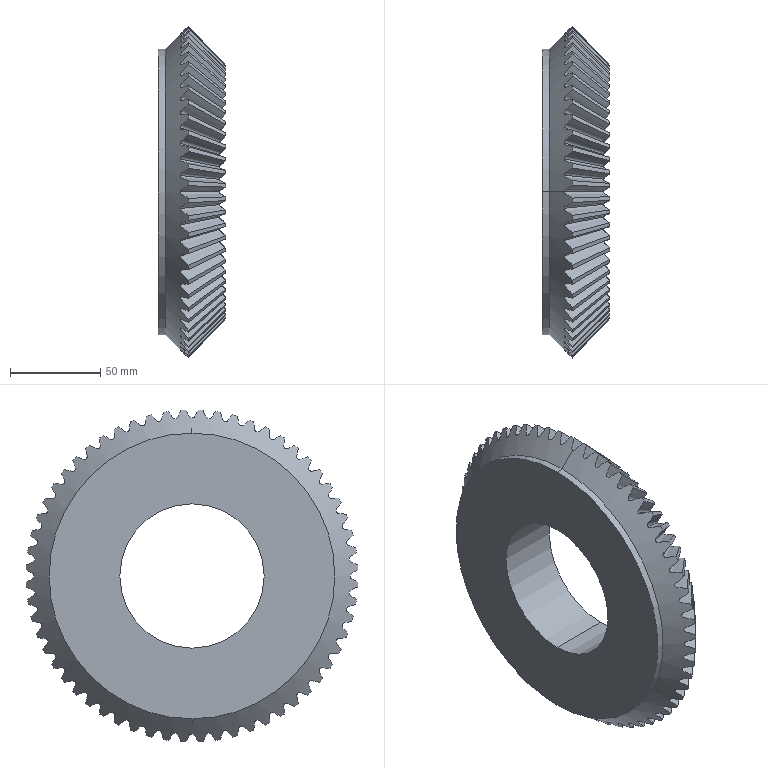Part | NX | features BREP 1 | 1 solid | 190 faces | box 37.656 x 184.108 x 184.108 mm | volume 545494 mm3 | spline 120 | cone 64 | cylinder 4 | plane 2 | commonest cylinder face diameters 80 x2 158.356 x2